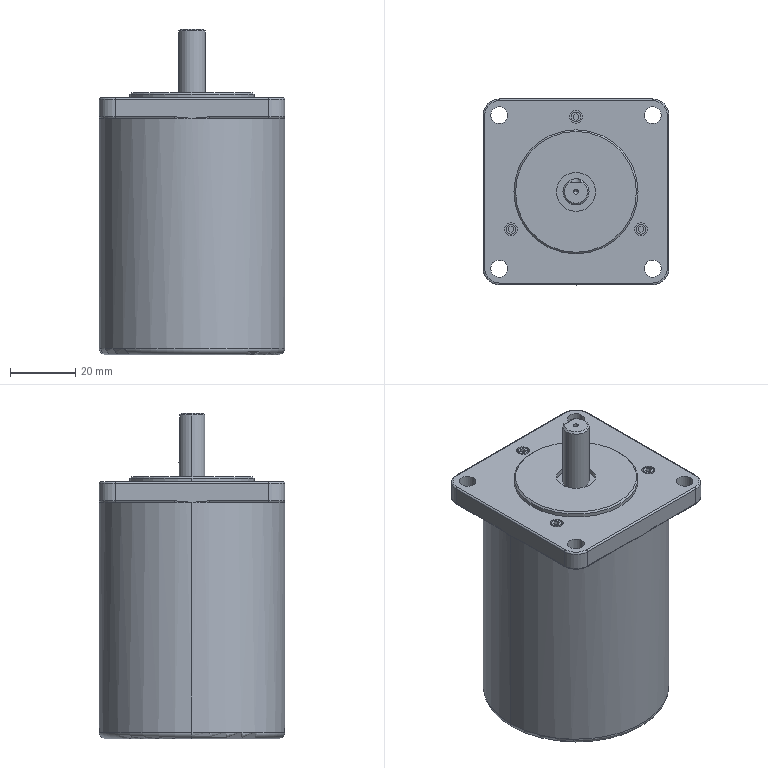Part | SolidWorks | features ICE 4, CirPattern 1, Fillet 1, LPattern 1, RevCut 1, Revolution 1, Sweep 1 | 1 solid | 115 faces | box 57 x 57 x 99.8 mm | volume 207235 mm3 | cylinder 47 | plane 43 | torus 10 | spline 8 | cone 7 | commonest cylinder face diameters 1 x12 5.2 x8 3 x7 4 x6 10 x4 1.5 x2